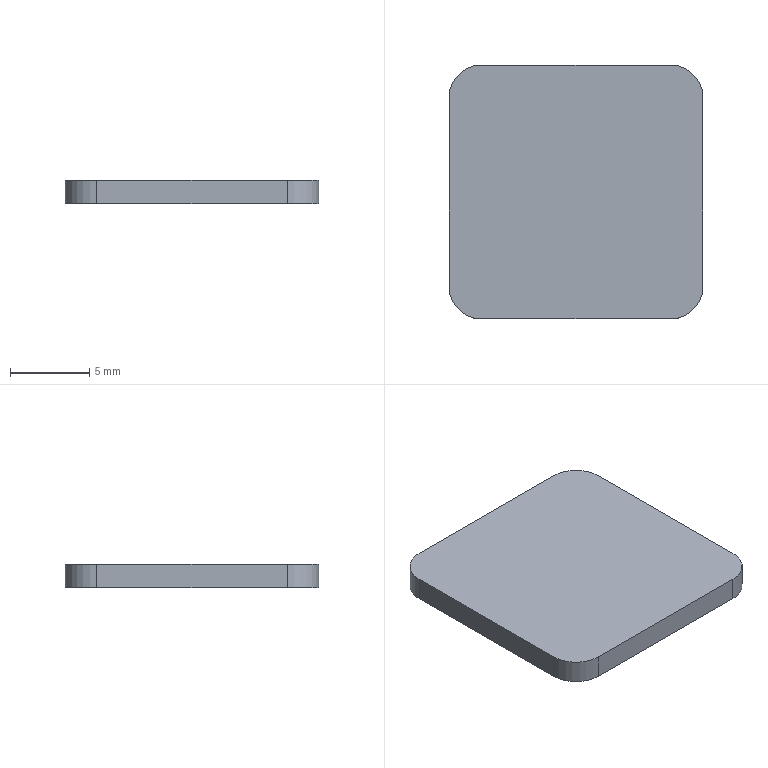Part | STEP file | KF-2212-070-003 | 1 solid | 10 faces | box 16 x 16 x 1.5 mm | volume 378.85 mm3 | plane 6 | cylinder 4 | commonest cylinder face diameters 4 x4
STEP:
#1=CARTESIAN_POINT('',(-6.,458.,0.));
#2=VERTEX_POINT('',#1);
#3=CARTESIAN_POINT('',(-8.,456.,0.));
#4=VERTEX_POINT('',#3);
#5=CARTESIAN_POINT('',(-6.,456.,0.));
#6=DIRECTION('',(0.,0.,1.));
#7=DIRECTION('',(1.,0.,0.));
#8=AXIS2_PLACEMENT_3D('',#5,#6,#7);
#9=CIRCLE('',#8,2.);
#10=EDGE_CURVE('',#2,#4,#9,.T.);
#11=ORIENTED_EDGE('',*,*,#10,.F.);
#12=CARTESIAN_POINT('',(-6.,458.,-1.5));
#13=VERTEX_POINT('',#12);
#14=CARTESIAN_POINT('',(-6.,458.,-1.5));
#15=DIRECTION('',(0.,0.,1.));
#16=VECTOR('',#15,1000.);
#17=LINE('',#14,#16);
#18=EDGE_CURVE('',#13,#2,#17,.T.);
#19=ORIENTED_EDGE('',*,*,#18,.F.);
#20=CARTESIAN_POINT('',(-8.,456.,-1.5));
#21=VERTEX_POINT('',#20);
#22=CARTESIAN_POINT('',(-6.,456.,-1.5));
#23=DIRECTION('',(0.,0.,1.));
#24=DIRECTION('',(1.,0.,0.));
#25=AXIS2_PLACEMENT_3D('',#22,#23,#24);
#26=CIRCLE('',#25,2.);
#27=EDGE_CURVE('',#13,#21,#26,.T.);
#28=ORIENTED_EDGE('',*,*,#27,.T.);
#29=CARTESIAN_POINT('',(-8.,456.,-1.5));
#30=DIRECTION('',(0.,0.,1.));
#31=VECTOR('',#30,1000.);
#32=LINE('',#29,#31);
#33=EDGE_CURVE('',#21,#4,#32,.T.);
#34=ORIENTED_EDGE('',*,*,#33,.T.);
#35=EDGE_LOOP('',(#11,#19,#28,#34));
#36=FACE_OUTER_BOUND('',#35,.T.);
#37=CARTESIAN_POINT('',(-6.,456.,-1.5));
#38=DIRECTION('',(0.,0.,1.));
#39=DIRECTION('',(1.,0.,0.));
#40=AXIS2_PLACEMENT_3D('',#37,#38,#39);
#41=CYLINDRICAL_SURFACE('',#40,2.);
#42=ADVANCED_FACE('',(#36),#41,.T.);
#43=CARTESIAN_POINT('',(6.,458.,0.));
#44=VERTEX_POINT('',#43);
#45=CARTESIAN_POINT('',(6.,458.,0.));
#46=DIRECTION('',(-1.,0.,0.));
#47=VECTOR('',#46,1000.);
#48=LINE('',#45,#47);
#49=EDGE_CURVE('',#44,#2,#48,.T.);
#50=ORIENTED_EDGE('',*,*,#49,.F.);
#51=CARTESIAN_POINT('',(6.,458.,-1.5));
#52=VERTEX_POINT('',#51);
#53=CARTESIAN_POINT('',(6.,458.,-1.5));
#54=DIRECTION('',(0.,0.,1.));
#55=VECTOR('',#54,1000.);
#56=LINE('',#53,#55);
#57=EDGE_CURVE('',#52,#44,#56,.T.);
#58=ORIENTED_EDGE('',*,*,#57,.F.);
#59=CARTESIAN_POINT('',(6.,458.,-1.5));
#60=DIRECTION('',(-1.,0.,0.));
#61=VECTOR('',#60,1000.);
#62=LINE('',#59,#61);
#63=EDGE_CURVE('',#52,#13,#62,.T.);
#64=ORIENTED_EDGE('',*,*,#63,.T.);
#65=ORIENTED_EDGE('',*,*,#18,.T.);
#66=EDGE_LOOP('',(#50,#58,#64,#65));
#67=FACE_OUTER_BOUND('',#66,.T.);
#68=CARTESIAN_POINT('',(6.,458.,-1.5));
#69=DIRECTION('',(0.,1.,0.));
#70=DIRECTION('',(0.,0.,1.));
#71=AXIS2_PLACEMENT_3D('',#68,#69,#70);
#72=PLANE('',#71);
#73=ADVANCED_FACE('',(#67),#72,.T.);
#74=CARTESIAN_POINT('',(8.,456.,0.));
#75=VERTEX_POINT('',#74);
#76=CARTESIAN_POINT('',(6.,456.,0.));
#77=DIRECTION('',(0.,0.,1.));
#78=DIRECTION('',(1.,0.,0.));
#79=AXIS2_PLACEMENT_3D('',#76,#77,#78);
#80=CIRCLE('',#79,2.);
#81=EDGE_CURVE('',#75,#44,#80,.T.);
#82=ORIENTED_EDGE('',*,*,#81,.F.);
#83=CARTESIAN_POINT('',(8.,456.,-1.5));
#84=VERTEX_POINT('',#83);
#85=CARTESIAN_POINT('',(8.,456.,-1.5));
#86=DIRECTION('',(0.,0.,1.));
#87=VECTOR('',#86,1000.);
#88=LINE('',#85,#87);
#89=EDGE_CURVE('',#84,#75,#88,.T.);
#90=ORIENTED_EDGE('',*,*,#89,.F.);
#91=CARTESIAN_POINT('',(6.,456.,-1.5));
#92=DIRECTION('',(0.,0.,1.));
#93=DIRECTION('',(1.,0.,0.));
#94=AXIS2_PLACEMENT_3D('',#91,#92,#93);
#95=CIRCLE('',#94,2.);
#96=EDGE_CURVE('',#84,#52,#95,.T.);
#97=ORIENTED_EDGE('',*,*,#96,.T.);
#98=ORIENTED_EDGE('',*,*,#57,.T.);
#99=EDGE_LOOP('',(#82,#90,#97,#98));
#100=FACE_OUTER_BOUND('',#99,.T.);
#101=CARTESIAN_POINT('',(6.,456.,-1.5));
#102=DIRECTION('',(0.,0.,1.));
#103=DIRECTION('',(1.,0.,0.));
#104=AXIS2_PLACEMENT_3D('',#101,#102,#103);
#105=CYLINDRICAL_SURFACE('',#104,2.);
#106=ADVANCED_FACE('',(#100),#105,.T.);
#107=CARTESIAN_POINT('',(8.,444.,0.));
#108=VERTEX_POINT('',#107);
#109=CARTESIAN_POINT('',(8.,444.,0.));
#110=DIRECTION('',(0.,1.,0.));
#111=VECTOR('',#110,1000.);
#112=LINE('',#109,#111);
#113=EDGE_CURVE('',#108,#75,#112,.T.);
#114=ORIENTED_EDGE('',*,*,#113,.F.);
#115=CARTESIAN_POINT('',(8.,444.,-1.5));
#116=VERTEX_POINT('',#115);
#117=CARTESIAN_POINT('',(8.,444.,-1.5));
#118=DIRECTION('',(0.,0.,1.));
#119=VECTOR('',#118,1000.);
#120=LINE('',#117,#119);
#121=EDGE_CURVE('',#116,#108,#120,.T.);
#122=ORIENTED_EDGE('',*,*,#121,.F.);
#123=CARTESIAN_POINT('',(8.,444.,-1.5));
#124=DIRECTION('',(0.,1.,0.));
#125=VECTOR('',#124,1000.);
#126=LINE('',#123,#125);
#127=EDGE_CURVE('',#116,#84,#126,.T.);
#128=ORIENTED_EDGE('',*,*,#127,.T.);
#129=ORIENTED_EDGE('',*,*,#89,.T.);
#130=EDGE_LOOP('',(#114,#122,#128,#129));
#131=FACE_OUTER_BOUND('',#130,.T.);
#132=CARTESIAN_POINT('',(8.,444.,-1.5));
#133=DIRECTION('',(1.,0.,0.));
#134=DIRECTION('',(0.,0.,-1.));
#135=AXIS2_PLACEMENT_3D('',#132,#133,#134);
#136=PLANE('',#135);
#137=ADVANCED_FACE('',(#131),#136,.T.);
#138=CARTESIAN_POINT('',(6.,442.,0.));
#139=VERTEX_POINT('',#138);
#140=CARTESIAN_POINT('',(6.,444.,0.));
#141=DIRECTION('',(0.,0.,1.));
#142=DIRECTION('',(1.,0.,0.));
#143=AXIS2_PLACEMENT_3D('',#140,#141,#142);
#144=CIRCLE('',#143,2.);
#145=EDGE_CURVE('',#139,#108,#144,.T.);
#146=ORIENTED_EDGE('',*,*,#145,.F.);
#147=CARTESIAN_POINT('',(6.,442.,-1.5));
#148=VERTEX_POINT('',#147);
#149=CARTESIAN_POINT('',(6.,442.,-1.5));
#150=DIRECTION('',(0.,0.,1.));
#151=VECTOR('',#150,1000.);
#152=LINE('',#149,#151);
#153=EDGE_CURVE('',#148,#139,#152,.T.);
#154=ORIENTED_EDGE('',*,*,#153,.F.);
#155=CARTESIAN_POINT('',(6.,444.,-1.5));
#156=DIRECTION('',(0.,0.,1.));
#157=DIRECTION('',(1.,0.,0.));
#158=AXIS2_PLACEMENT_3D('',#155,#156,#157);
#159=CIRCLE('',#158,2.);
#160=EDGE_CURVE('',#148,#116,#159,.T.);
#161=ORIENTED_EDGE('',*,*,#160,.T.);
#162=ORIENTED_EDGE('',*,*,#121,.T.);
#163=EDGE_LOOP('',(#146,#154,#161,#162));
#164=FACE_OUTER_BOUND('',#163,.T.);
#165=CARTESIAN_POINT('',(6.,444.,-1.5));
#166=DIRECTION('',(0.,0.,1.));
#167=DIRECTION('',(1.,0.,0.));
#168=AXIS2_PLACEMENT_3D('',#165,#166,#167);
#169=CYLINDRICAL_SURFACE('',#168,2.);
#170=ADVANCED_FACE('',(#164),#169,.T.);
#171=CARTESIAN_POINT('',(-6.,442.,0.));
#172=VERTEX_POINT('',#171);
#173=CARTESIAN_POINT('',(-6.,442.,0.));
#174=DIRECTION('',(1.,0.,0.));
#175=VECTOR('',#174,1000.);
#176=LINE('',#173,#175);
#177=EDGE_CURVE('',#172,#139,#176,.T.);
#178=ORIENTED_EDGE('',*,*,#177,.F.);
#179=CARTESIAN_POINT('',(-6.,442.,-1.5));
#180=VERTEX_POINT('',#179);
#181=CARTESIAN_POINT('',(-6.,442.,-1.5));
#182=DIRECTION('',(0.,0.,1.));
#183=VECTOR('',#182,1000.);
#184=LINE('',#181,#183);
#185=EDGE_CURVE('',#180,#172,#184,.T.);
#186=ORIENTED_EDGE('',*,*,#185,.F.);
#187=CARTESIAN_POINT('',(-6.,442.,-1.5));
#188=DIRECTION('',(1.,0.,0.));
#189=VECTOR('',#188,1000.);
#190=LINE('',#187,#189);
#191=EDGE_CURVE('',#180,#148,#190,.T.);
#192=ORIENTED_EDGE('',*,*,#191,.T.);
#193=ORIENTED_EDGE('',*,*,#153,.T.);
#194=EDGE_LOOP('',(#178,#186,#192,#193));
#195=FACE_OUTER_BOUND('',#194,.T.);
#196=CARTESIAN_POINT('',(-6.,442.,-1.5));
#197=DIRECTION('',(0.,-1.,0.));
#198=DIRECTION('',(0.,0.,-1.));
#199=AXIS2_PLACEMENT_3D('',#196,#197,#198);
#200=PLANE('',#199);
#201=ADVANCED_FACE('',(#195),#200,.T.);
#202=CARTESIAN_POINT('',(-8.,444.,0.));
#203=VERTEX_POINT('',#202);
#204=CARTESIAN_POINT('',(-6.,444.,0.));
#205=DIRECTION('',(0.,0.,1.));
#206=DIRECTION('',(1.,0.,0.));
#207=AXIS2_PLACEMENT_3D('',#204,#205,#206);
#208=CIRCLE('',#207,2.);
#209=EDGE_CURVE('',#203,#172,#208,.T.);
#210=ORIENTED_EDGE('',*,*,#209,.F.);
#211=CARTESIAN_POINT('',(-8.,444.,-1.5));
#212=VERTEX_POINT('',#211);
#213=CARTESIAN_POINT('',(-8.,444.,-1.5));
#214=DIRECTION('',(0.,0.,1.));
#215=VECTOR('',#214,1000.);
#216=LINE('',#213,#215);
#217=EDGE_CURVE('',#212,#203,#216,.T.);
#218=ORIENTED_EDGE('',*,*,#217,.F.);
#219=CARTESIAN_POINT('',(-6.,444.,-1.5));
#220=DIRECTION('',(0.,0.,1.));
#221=DIRECTION('',(1.,0.,0.));
#222=AXIS2_PLACEMENT_3D('',#219,#220,#221);
#223=CIRCLE('',#222,2.);
#224=EDGE_CURVE('',#212,#180,#223,.T.);
#225=ORIENTED_EDGE('',*,*,#224,.T.);
#226=ORIENTED_EDGE('',*,*,#185,.T.);
#227=EDGE_LOOP('',(#210,#218,#225,#226));
#228=FACE_OUTER_BOUND('',#227,.T.);
#229=CARTESIAN_POINT('',(-6.,444.,-1.5));
#230=DIRECTION('',(0.,0.,1.));
#231=DIRECTION('',(1.,0.,0.));
#232=AXIS2_PLACEMENT_3D('',#229,#230,#231);
#233=CYLINDRICAL_SURFACE('',#232,2.);
#234=ADVANCED_FACE('',(#228),#233,.T.);
#235=CARTESIAN_POINT('',(-8.,456.,0.));
#236=DIRECTION('',(0.,-1.,0.));
#237=VECTOR('',#236,1000.);
#238=LINE('',#235,#237);
#239=EDGE_CURVE('',#4,#203,#238,.T.);
#240=ORIENTED_EDGE('',*,*,#239,.F.);
#241=ORIENTED_EDGE('',*,*,#33,.F.);
#242=CARTESIAN_POINT('',(-8.,456.,-1.5));
#243=DIRECTION('',(0.,-1.,0.));
#244=VECTOR('',#243,1000.);
#245=LINE('',#242,#244);
#246=EDGE_CURVE('',#21,#212,#245,.T.);
#247=ORIENTED_EDGE('',*,*,#246,.T.);
#248=ORIENTED_EDGE('',*,*,#217,.T.);
#249=EDGE_LOOP('',(#240,#241,#247,#248));
#250=FACE_OUTER_BOUND('',#249,.T.);
#251=CARTESIAN_POINT('',(-8.,456.,-1.5));
#252=DIRECTION('',(-1.,0.,0.));
#253=DIRECTION('',(0.,0.,1.));
#254=AXIS2_PLACEMENT_3D('',#251,#252,#253);
#255=PLANE('',#254);
#256=ADVANCED_FACE('',(#250),#255,.T.);
#257=ORIENTED_EDGE('',*,*,#27,.F.);
#258=ORIENTED_EDGE('',*,*,#63,.F.);
#259=ORIENTED_EDGE('',*,*,#96,.F.);
#260=ORIENTED_EDGE('',*,*,#127,.F.);
#261=ORIENTED_EDGE('',*,*,#160,.F.);
#262=ORIENTED_EDGE('',*,*,#191,.F.);
#263=ORIENTED_EDGE('',*,*,#224,.F.);
#264=ORIENTED_EDGE('',*,*,#246,.F.);
#265=EDGE_LOOP('',(#257,#258,#259,#260,#261,#262,#263,#264));
#266=FACE_OUTER_BOUND('',#265,.T.);
#267=CARTESIAN_POINT('',(-6.,456.,-1.5));
#268=DIRECTION('',(0.,0.,1.));
#269=DIRECTION('',(1.,0.,0.));
#270=AXIS2_PLACEMENT_3D('',#267,#268,#269);
#271=PLANE('',#270);
#272=ADVANCED_FACE('',(#266),#271,.F.);
#273=ORIENTED_EDGE('',*,*,#10,.T.);
#274=ORIENTED_EDGE('',*,*,#239,.T.);
#275=ORIENTED_EDGE('',*,*,#209,.T.);
#276=ORIENTED_EDGE('',*,*,#177,.T.);
#277=ORIENTED_EDGE('',*,*,#145,.T.);
#278=ORIENTED_EDGE('',*,*,#113,.T.);
#279=ORIENTED_EDGE('',*,*,#81,.T.);
#280=ORIENTED_EDGE('',*,*,#49,.T.);
#281=EDGE_LOOP('',(#273,#274,#275,#276,#277,#278,#279,#280));
#282=FACE_OUTER_BOUND('',#281,.T.);
#283=CARTESIAN_POINT('',(-6.,456.,0.));
#284=DIRECTION('',(0.,0.,1.));
#285=DIRECTION('',(1.,0.,0.));
#286=AXIS2_PLACEMENT_3D('',#283,#284,#285);
#287=PLANE('',#286);
#288=ADVANCED_FACE('',(#282),#287,.T.);
#289=CLOSED_SHELL('',(#42,#73,#106,#137,#170,#201,#234,#256,#272,#288));
#290=MANIFOLD_SOLID_BREP('',#289);
#291=CARTESIAN_POINT('',(0.,0.,0.));
#292=DIRECTION('',(0.,0.,1.));
#293=DIRECTION('',(1.,0.,0.));
#294=AXIS2_PLACEMENT_3D('',#291,#292,#293);
#295=(LENGTH_UNIT()NAMED_UNIT(*)SI_UNIT(.MILLI.,.METRE.));
#296=UNCERTAINTY_MEASURE_WITH_UNIT(LENGTH_MEASURE(0.00001),#295,'','');
#297=(NAMED_UNIT(*)PLANE_ANGLE_UNIT()SI_UNIT($,.RADIAN.));
#298=(NAMED_UNIT(*)SI_UNIT($,.STERADIAN.)SOLID_ANGLE_UNIT());
#299=(GEOMETRIC_REPRESENTATION_CONTEXT(3)GLOBAL_UNCERTAINTY_ASSIGNED_CONTEXT((#296))GLOBAL_UNIT_ASSIGNED_CONTEXT((#295,#297,#298))REPRESENTATION_CONTEXT('',''));
#300=ADVANCED_BREP_SHAPE_REPRESENTATION('',(#290,#294),#299);